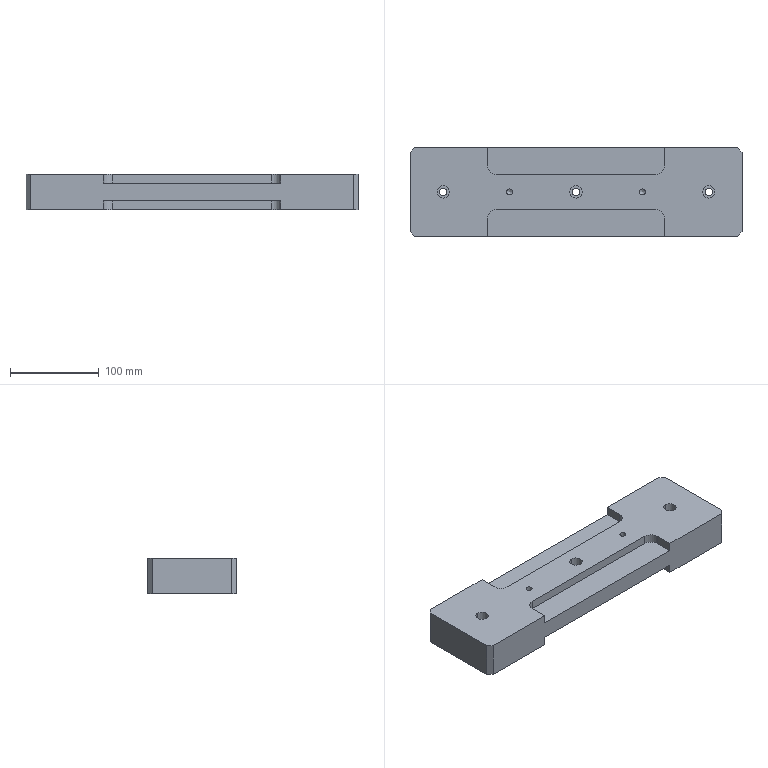NC program | NX | posted with a generic post | part box 375 x 100 x 40 mm
Whole program:
N10 G17 G21 G94 G90
(FLOOR_WALL_COPY , TOOL : D17R0.8)
N12 T21 M6
N14 G54
N16 G17 G0 G90 X6.755 Y-60. S2000 M3
N18 G43 Z30. H21
N20 Z1.17
N22 G94 G1 Z-0.33 F1000.
N24 X1.472 Y-50.85
N26 G3 X0. Y-50. R1.7
N28 G1 X-91.35 F2000.
N30 Y-30.
N32 G2 X-90. Y-28.65 R1.35
N34 G1 X90.
N36 G2 X91.35 Y-30. R1.35
N38 G1 Y-50.
N40 X0.
N42 Y-41.5
N44 X-82.85
N46 Y-37.15
N48 X82.85
N50 Y-41.5
N52 X0.
N54 G3 X-1.472 Y-42.35 R1.7
N56 G1 Z1.17
N58 G0 X6.755 Y-60. Z0.84
N60 G1 Z-0.66 F1000.
N62 X1.472 Y-50.85
N64 G3 X0. Y-50. R1.7
N66 G1 X-91.35 F2000.
N68 Y-30.
N70 G2 X-90. Y-28.65 R1.35
N72 G1 X90.
N74 G2 X91.35 Y-30. R1.35
N76 G1 Y-50.
N78 X0.
N80 Y-41.5
N82 X-82.85
N84 Y-37.15
N86 X82.85
N88 Y-41.5
N90 X0.
N92 G3 X-1.472 Y-42.35 R1.7
N94 G1 Z0.84
N96 G0 X6.755 Y-60. Z0.51
N98 G1 Z-0.99 F1000.
N100 X1.472 Y-50.85
N102 G3 X0. Y-50. R1.7
N104 G1 X-91.35 F2000.
N106 Y-30.
N108 G2 X-90. Y-28.65 R1.35
N110 G1 X90.
N112 G2 X91.35 Y-30. R1.35
N114 G1 Y-50.
N116 X0.
N118 Y-41.5
N120 X-82.85
N122 Y-37.15
N124 X82.85
N126 Y-41.5
N128 X0.
N130 G3 X-1.472 Y-42.35 R1.7
N132 G1 Z0.51
N134 G0 X6.755 Y-60. Z0.18
N136 G1 Z-1.32 F1000.
N138 X1.472 Y-50.85
N140 G3 X0. Y-50. R1.7
N142 G1 X-91.35 F2000.
N144 Y-30.
N146 G2 X-90. Y-28.65 R1.35
N148 G1 X90.
N150 G2 X91.35 Y-30. R1.35
N152 G1 Y-50.
N154 X0.
N156 Y-41.5
N158 X-82.85
N160 Y-37.15
N162 X82.85
N164 Y-41.5
N166 X0.
N168 G3 X-1.472 Y-42.35 R1.7
N170 G1 Z0.18
N172 G0 X6.755 Y-60. Z-0.15
N174 G1 Z-1.65 F1000.
N176 X1.472 Y-50.85
N178 G3 X0. Y-50. R1.7
N180 G1 X-91.35 F2000.
N182 Y-30.
N184 G2 X-90. Y-28.65 R1.35
N186 G1 X90.
N188 G2 X91.35 Y-30. R1.35
N190 G1 Y-50.
N192 X0.
N194 Y-41.5
N196 X-82.85
N198 Y-37.15
N200 X82.85
N202 Y-41.5
N204 X0.
N206 G3 X-1.472 Y-42.35 R1.7
N208 G1 Z-0.15
N210 G0 X6.755 Y-60. Z-0.48
N212 G1 Z-1.98 F1000.
N214 X1.472 Y-50.85
N216 G3 X0. Y-50. R1.7
N218 G1 X-91.35 F2000.
N220 Y-30.
N222 G2 X-90. Y-28.65 R1.35
N224 G1 X90.
N226 G2 X91.35 Y-30. R1.35
N228 G1 Y-50.
N230 X0.
N232 Y-41.5
N234 X-82.85
N236 Y-37.15
N238 X82.85
N240 Y-41.5
N242 X0.
N244 G3 X-1.472 Y-42.35 R1.7
N246 G1 Z-0.48
N248 G0 X6.755 Y-60. Z-0.81
N250 G1 Z-2.31 F1000.
N252 X1.472 Y-50.85
N254 G3 X0. Y-50. R1.7
N256 G1 X-91.35 F2000.
N258 Y-30.
N260 G2 X-90. Y-28.65 R1.35
N262 G1 X90.
N264 G2 X91.35 Y-30. R1.35
N266 G1 Y-50.
N268 X0.
N270 Y-41.5
N272 X-82.85
N274 Y-37.15
N276 X82.85
N278 Y-41.5
N280 X0.
N282 G3 X-1.472 Y-42.35 R1.7
N284 G1 Z-0.81
N286 G0 X6.755 Y-60. Z-1.14
N288 G1 Z-2.64 F1000.
N290 X1.472 Y-50.85
N292 G3 X0. Y-50. R1.7
N294 G1 X-91.35 F2000.
N296 Y-30.
N298 G2 X-90. Y-28.65 R1.35
N300 G1 X90.
N302 G2 X91.35 Y-30. R1.35
N304 G1 Y-50.
N306 X0.
N308 Y-41.5
N310 X-82.85
N312 Y-37.15
N314 X82.85
N316 Y-41.5
N318 X0.
N320 G3 X-1.472 Y-42.35 R1.7
N322 G1 Z-1.14
N324 G0 X6.755 Y-60. Z-1.47
N326 G1 Z-2.97 F1000.
N328 X1.472 Y-50.85
N330 G3 X0. Y-50. R1.7
N332 G1 X-91.35 F2000.
N334 Y-30.
N336 G2 X-90. Y-28.65 R1.35
N338 G1 X90.
N340 G2 X91.35 Y-30. R1.35
N342 G1 Y-50.
N344 X0.
N346 Y-41.5
N348 X-82.85
N350 Y-37.15
N352 X82.85
N354 Y-41.5
N356 X0.
N358 G3 X-1.472 Y-42.35 R1.7
N360 G1 Z-1.47
N362 G0 X6.755 Y-60. Z-1.8
N364 G1 Z-3.3 F1000.
N366 X1.472 Y-50.85
N368 G3 X0. Y-50. R1.7
N370 G1 X-91.35 F2000.
N372 Y-30.
N374 G2 X-90. Y-28.65 R1.35
N376 G1 X90.
N378 G2 X91.35 Y-30. R1.35
N380 G1 Y-50.
N382 X0.
N384 Y-41.5
N386 X-82.85
N388 Y-37.15
N390 X82.85
N392 Y-41.5
N394 X0.
N396 G3 X-1.472 Y-42.35 R1.7
N398 G1 Z-1.8
N400 G0 X6.755 Y-60. Z-2.13
N402 G1 Z-3.63 F1000.
N404 X1.472 Y-50.85
N406 G3 X0. Y-50. R1.7
N408 G1 X-91.35 F2000.
N410 Y-30.
N412 G2 X-90. Y-28.65 R1.35
N414 G1 X90.
N416 G2 X91.35 Y-30. R1.35
N418 G1 Y-50.
N420 X0.
N422 Y-41.5
N424 X-82.85
N426 Y-37.15
N428 X82.85
N430 Y-41.5
N432 X0.
N434 G3 X-1.472 Y-42.35 R1.7
N436 G1 Z-2.13
N438 G0 X6.755 Y-60. Z-2.46
N440 G1 Z-3.96 F1000.
N442 X1.472 Y-50.85
N444 G3 X0. Y-50. R1.7
N446 G1 X-91.35 F2000.
N448 Y-30.
N450 G2 X-90. Y-28.65 R1.35
N452 G1 X90.
N454 G2 X91.35 Y-30. R1.35
N456 G1 Y-50.
N458 X0.
N460 Y-41.5
N462 X-82.85
N464 Y-37.15
N466 X82.85
N468 Y-41.5
N470 X0.
N472 G3 X-1.472 Y-42.35 R1.7
N474 G1 Z-2.46
N476 G0 X6.755 Y-60. Z-2.79
N478 G1 Z-4.29 F1000.
N480 X1.472 Y-50.85
N482 G3 X0. Y-50. R1.7
N484 G1 X-91.35 F2000.
N486 Y-30.
N488 G2 X-90. Y-28.65 R1.35
N490 G1 X90.
N492 G2 X91.35 Y-30. R1.35
N494 G1 Y-50.
N496 X0.
N498 Y-41.5
N500 X-82.85
N502 Y-37.15
N504 X82.85
N506 Y-41.5
N508 X0.
N510 G3 X-1.472 Y-42.35 R1.7
N512 G1 Z-2.79
N514 G0 X6.755 Y-60. Z-3.12
N516 G1 Z-4.62 F1000.
N518 X1.472 Y-50.85
N520 G3 X0. Y-50. R1.7
N522 G1 X-91.35 F2000.
N524 Y-30.
N526 G2 X-90. Y-28.65 R1.35
N528 G1 X90.
N530 G2 X91.35 Y-30. R1.35
N532 G1 Y-50.
N534 X0.
N536 Y-41.5
N538 X-82.85
N540 Y-37.15
N542 X82.85
N544 Y-41.5
N546 X0.
N548 G3 X-1.472 Y-42.35 R1.7
N550 G1 Z-3.12
N552 G0 X6.755 Y-60. Z-3.45
N554 G1 Z-4.95 F1000.
N556 X1.472 Y-50.85
N558 G3 X0. Y-50. R1.7
N560 G1 X-91.35 F2000.
N562 Y-30.
N564 G2 X-90. Y-28.65 R1.35
N566 G1 X90.
N568 G2 X91.35 Y-30. R1.35
N570 G1 Y-50.
N572 X0.
N574 Y-41.5
N576 X-82.85
N578 Y-37.15
N580 X82.85
N582 Y-41.5
N584 X0.
N586 G3 X-1.472 Y-42.35 R1.7
N588 G1 Z-3.45
N590 G0 X6.755 Y-60. Z-3.78
N592 G1 Z-5.28 F1000.
N594 X1.472 Y-50.85
N596 G3 X0. Y-50. R1.7
N598 G1 X-91.35 F2000.
N600 Y-30.
N602 G2 X-90. Y-28.65 R1.35
N604 G1 X90.
N606 G2 X91.35 Y-30. R1.35
N608 G1 Y-50.
N610 X0.
N612 Y-41.5
N614 X-82.85
N616 Y-37.15
N618 X82.85
N620 Y-41.5
N622 X0.
N624 G3 X-1.472 Y-42.35 R1.7
N626 G1 Z-3.78
N628 G0 X6.755 Y-60. Z-4.11
N630 G1 Z-5.61 F1000.
N632 X1.472 Y-50.85
N634 G3 X0. Y-50. R1.7
N636 G1 X-91.35 F2000.
N638 Y-30.
N640 G2 X-90. Y-28.65 R1.35
N642 G1 X90.
N644 G2 X91.35 Y-30. R1.35
N646 G1 Y-50.
N648 X0.
N650 Y-41.5
N652 X-82.85
N654 Y-37.15
N656 X82.85
N658 Y-41.5
N660 X0.
N662 G3 X-1.472 Y-42.35 R1.7
N664 G1 Z-4.11
N666 G0 X6.755 Y-60. Z-4.44
N668 G1 Z-5.94 F1000.
N670 X1.472 Y-50.85
N672 G3 X0. Y-50. R1.7
N674 G1 X-91.35 F2000.
N676 Y-30.
N678 G2 X-90. Y-28.65 R1.35
N680 G1 X90.
N682 G2 X91.35 Y-30. R1.35
N684 G1 Y-50.
N686 X0.
N688 Y-41.5
N690 X-82.85
N692 Y-37.15
N694 X82.85
N696 Y-41.5
N698 X0.
N700 G3 X-1.472 Y-42.35 R1.7
N702 G1 Z-4.44
N704 G0 X6.755 Y-60. Z-4.77
N706 G1 Z-6.27 F1000.
N708 X1.472 Y-50.85
N710 G3 X0. Y-50. R1.7
N712 G1 X-91.35 F2000.
N714 Y-30.
N716 G2 X-90. Y-28.65 R1.35
N718 G1 X90.
N720 G2 X91.35 Y-30. R1.35
N722 G1 Y-50.
N724 X0.
N726 Y-41.5
N728 X-82.85
N730 Y-37.15
N732 X82.85
N734 Y-41.5
N736 X0.
N738 G3 X-1.472 Y-42.35 R1.7
N740 G1 Z-4.77
N742 G0 X6.755 Y-60. Z-5.1
N744 G1 Z-6.6 F1000.
N746 X1.472 Y-50.85
N748 G3 X0. Y-50. R1.7
N750 G1 X-91.35 F2000.
N752 Y-30.
N754 G2 X-90. Y-28.65 R1.35
N756 G1 X90.
N758 G2 X91.35 Y-30. R1.35
N760 G1 Y-50.
N762 X0.
N764 Y-41.5
N766 X-82.85
N768 Y-37.15
N770 X82.85
N772 Y-41.5
N774 X0.
N776 G3 X-1.472 Y-42.35 R1.7
N778 G1 Z-5.1
N780 G0 X6.755 Y-60. Z-5.43
N782 G1 Z-6.93 F1000.
N784 X1.472 Y-50.85
N786 G3 X0. Y-50. R1.7
N788 G1 X-91.35 F2000.
N790 Y-30.
N792 G2 X-90. Y-28.65 R1.35
N794 G1 X90.
N796 G2 X91.35 Y-30. R1.35
N798 G1 Y-50.
N800 X0.
N802 Y-41.5
N804 X-82.85
N806 Y-37.15
N808 X82.85
N810 Y-41.5
N812 X0.
N814 G3 X-1.472 Y-42.35 R1.7
N816 G1 Z-5.43
N818 G0 X6.755 Y-60. Z-5.76
N820 G1 Z-7.26 F1000.
N822 X1.472 Y-50.85
N824 G3 X0. Y-50. R1.7
N826 G1 X-91.35 F2000.
N828 Y-30.
N830 G2 X-90. Y-28.65 R1.35
N832 G1 X90.
N834 G2 X91.35 Y-30. R1.35
N836 G1 Y-50.
N838 X0.
N840 Y-41.5
N842 X-82.85
N844 Y-37.15
N846 X82.85
N848 Y-41.5
N850 X0.
N852 G3 X-1.472 Y-42.35 R1.7
N854 G1 Z-5.76
N856 G0 X6.755 Y-60. Z-6.09
N858 G1 Z-7.59 F1000.
N860 X1.472 Y-50.85
N862 G3 X0. Y-50. R1.7
N864 G1 X-91.35 F2000.
N866 Y-30.
N868 G2 X-90. Y-28.65 R1.35
N870 G1 X90.
N872 G2 X91.35 Y-30. R1.35
N874 G1 Y-50.
N876 X0.
N878 Y-41.5
N880 X-82.85
N882 Y-37.15
N884 X82.85
N886 Y-41.5
N888 X0.
N890 G3 X-1.472 Y-42.35 R1.7
N892 G1 Z-6.09
N894 G0 X6.755 Y-60. Z-6.42
N896 G1 Z-7.92 F1000.
N898 X1.472 Y-50.85
N900 G3 X0. Y-50. R1.7
N902 G1 X-91.35 F2000.
N904 Y-30.
N906 G2 X-90. Y-28.65 R1.35
N908 G1 X90.
N910 G2 X91.35 Y-30. R1.35
N912 G1 Y-50.
N914 X0.
N916 Y-41.5
N918 X-82.85
N920 Y-37.15
N922 X82.85
N924 Y-41.5
N926 X0.
N928 G3 X-1.472 Y-42.35 R1.7
N930 G1 Z-6.42
N932 G0 X6.755 Y-60. Z-6.75
N934 G1 Z-8.25 F1000.
N936 X1.472 Y-50.85
N938 G3 X0. Y-50. R1.7
N940 G1 X-91.35 F2000.
N942 Y-30.
N944 G2 X-90. Y-28.65 R1.35
N946 G1 X90.
N948 G2 X91.35 Y-30. R1.35
N950 G1 Y-50.
N952 X0.
N954 Y-41.5
N956 X-82.85
N958 Y-37.15
N960 X82.85
N962 Y-41.5
N964 X0.
N966 G3 X-1.472 Y-42.35 R1.7
N968 G1 Z-6.75
N970 G0 X6.755 Y-60. Z-7.08
N972 G1 Z-8.58 F1000.
N974 X1.472 Y-50.85
N976 G3 X0. Y-50. R1.7
N978 G1 X-91.35 F2000.
N980 Y-30.
N982 G2 X-90. Y-28.65 R1.35
N984 G1 X90.
N986 G2 X91.35 Y-30. R1.35
N988 G1 Y-50.
N990 X0.
N992 Y-41.5
N994 X-82.85
N996 Y-37.15
N998 X82.85
N1000 Y-41.5
N1002 X0.
N1004 G3 X-1.472 Y-42.35 R1.7
N1006 G1 Z-7.08
N1008 G0 X6.755 Y-60. Z-7.41
N1010 G1 Z-8.91 F1000.
N1012 X1.472 Y-50.85
N1014 G3 X0. Y-50. R1.7
N1016 G1 X-91.35 F2000.
N1018 Y-30.
N1020 G2 X-90. Y-28.65 R1.35
N1022 G1 X90.
N1024 G2 X91.35 Y-30. R1.35
N1026 G1 Y-50.
N1028 X0.
N1030 Y-41.5
N1032 X-82.85
N1034 Y-37.15
N1036 X82.85
N1038 Y-41.5
N1040 X0.
N1042 G3 X-1.472 Y-42.35 R1.7
N1044 G1 Z-7.41
N1046 G0 X6.755 Y-60. Z-7.74
N1048 G1 Z-9.24 F1000.
N1050 X1.472 Y-50.85
N1052 G3 X0. Y-50. R1.7
N1054 G1 X-91.35 F2000.
N1056 Y-30.
N1058 G2 X-90. Y-28.65 R1.35
N1060 G1 X90.
N1062 G2 X91.35 Y-30. R1.35
N1064 G1 Y-50.
N1066 X0.
N1068 Y-41.5
N1070 X-82.85
N1072 Y-37.15
N1074 X82.85
N1076 Y-41.5
N1078 X0.
N1080 G3 X-1.472 Y-42.35 R1.7
N1082 G1 Z-7.74
N1084 G0 X6.755 Y-60. Z-8.07
N1086 G1 Z-9.57 F1000.
N1088 X1.472 Y-50.85
N1090 G3 X0. Y-50. R1.7
N1092 G1 X-91.35 F2000.
N1094 Y-30.
N1096 G2 X-90. Y-28.65 R1.35
N1098 G1 X90.
N1100 G2 X91.35 Y-30. R1.35
N1102 G1 Y-50.
N1104 X0.
N1106 Y-41.5
N1108 X-82.85
N1110 Y-37.15
N1112 X82.85
N1114 Y-41.5
N1116 X0.
N1118 G3 X-1.472 Y-42.35 R1.7
N1120 G1 Z-8.07
N1122 G0 X6.755 Y-60. Z-8.4
N1124 G1 Z-9.9 F1000.
N1126 X1.472 Y-50.85
N1128 G3 X0. Y-50. R1.7
N1130 G1 X-91.35 F2000.
N1132 Y-30.
N1134 G2 X-90. Y-28.65 R1.35
N1136 G1 X90.
N1138 G2 X91.35 Y-30. R1.35
N1140 G1 Y-50.
N1142 X0.
N1144 Y-41.5
N1146 X-82.85
N1148 Y-37.15
N1150 X82.85
N1152 Y-41.5
N1154 X0.
N1156 G3 X-1.472 Y-42.35 R1.7
N1158 G1 Z-8.4
N1160 G0 Z30.
N1162 X-6.755 Y60.
N1164 Z1.17
N1166 G1 Z-0.33 F1000.
N1168 X-1.472 Y50.85
N1170 G3 X0. Y50. R1.7
N1172 G1 X91.35 F2000.
N1174 Y30.
N1176 G2 X90. Y28.65 R1.35
N1178 G1 X-90.
N1180 G2 X-91.35 Y30. R1.35
N1182 G1 Y50.
N1184 X0.
N1186 Y41.5
N1188 X82.85
N1190 Y37.15
N1192 X-82.85
N1194 Y41.5
N1196 X0.
N1198 G3 X1.472 Y42.35 R1.7
N1200 G1 Z1.17
N1202 G0 X-6.755 Y60. Z0.84
N1204 G1 Z-0.66 F1000.
N1206 X-1.472 Y50.85
N1208 G3 X0. Y50. R1.7
N1210 G1 X91.35 F2000.
N1212 Y30.
N1214 G2 X90. Y28.65 R1.35
N1216 G1 X-90.
N1218 G2 X-91.35 Y30. R1.35
N1220 G1 Y50.
N1222 X0.
N1224 Y41.5
N1226 X82.85
N1228 Y37.15
N1230 X-82.85
N1232 Y41.5
N1234 X0.
N1236 G3 X1.472 Y42.35 R1.7
N1238 G1 Z0.84
N1240 G0 X-6.755 Y60. Z0.51
N1242 G1 Z-0.99 F1000.
N1244 X-1.472 Y50.85
N1246 G3 X0. Y50. R1.7
N1248 G1 X91.35 F2000.
N1250 Y30.
N1252 G2 X90. Y28.65 R1.35
N1254 G1 X-90.
N1256 G2 X-91.35 Y30. R1.35
N1258 G1 Y50.
N1260 X0.
N1262 Y41.5
N1264 X82.85
N1266 Y37.15
N1268 X-82.85
N1270 Y41.5
N1272 X0.
N1274 G3 X1.472 Y42.35 R1.7
N1276 G1 Z0.51
N1278 G0 X-6.755 Y60. Z0.18
N1280 G1 Z-1.32 F1000.
N1282 X-1.472 Y50.85
N1284 G3 X0. Y50. R1.7
N1286 G1 X91.35 F2000.
N1288 Y30.
N1290 G2 X90. Y28.65 R1.35
N1292 G1 X-90.
N1294 G2 X-91.35 Y30. R1.35
N1296 G1 Y50.
N1298 X0.
N1300 Y41.5
N1302 X82.85
N1304 Y37.15
N1306 X-82.85
N1308 Y41.5
N1310 X0.
N1312 G3 X1.472 Y42.35 R1.7
N1314 G1 Z0.18
N1316 G0 X-6.755 Y60. Z-0.15
N1318 G1 Z-1.65 F1000.
N1320 X-1.472 Y50.85
N1322 G3 X0. Y50. R1.7
N1324 G1 X91.35 F2000.
N1326 Y30.
N1328 G2 X90. Y28.65 R1.35
N1330 G1 X-90.
N1332 G2 X-91.35 Y30. R1.35
N1334 G1 Y50.
N1336 X0.
N1338 Y41.5
N1340 X82.85
N1342 Y37.15
N1344 X-82.85
N1346 Y41.5
N1348 X0.
N1350 G3 X1.472 Y42.35 R1.7
N1352 G1 Z-0.15
N1354 G0 X-6.755 Y60. Z-0.48
N1356 G1 Z-1.98 F1000.
N1358 X-1.472 Y50.85
N1360 G3 X0. Y50. R1.7
N1362 G1 X91.35 F2000.
N1364 Y30.
N1366 G2 X90. Y28.65 R1.35
N1368 G1 X-90.
N1370 G2 X-91.35 Y30. R1.35
N1372 G1 Y50.
N1374 X0.
N1376 Y41.5
N1378 X82.85
N1380 Y37.15
N1382 X-82.85
N1384 Y41.5
N1386 X0.
N1388 G3 X1.472 Y42.35 R1.7
N1390 G1 Z-0.48
N1392 G0 X-6.755 Y60. Z-0.81
N1394 G1 Z-2.31 F1000.
N1396 X-1.472 Y50.85
N1398 G3 X0. Y50. R1.7
N1400 G1 X91.35 F2000.
N1402 Y30.
N1404 G2 X90. Y28.65 R1.35
N1406 G1 X-90.
N1408 G2 X-91.35 Y30. R1.35
N1410 G1 Y50.
N1412 X0.
N1414 Y41.5
N1416 X82.85
N1418 Y37.15
N1420 X-82.85
N1422 Y41.5
N1424 X0.
N1426 G3 X1.472 Y42.35 R1.7
N1428 G1 Z-0.81
N1430 G0 X-6.755 Y60. Z-1.14
N1432 G1 Z-2.64 F1000.
N1434 X-1.472 Y50.85
N1436 G3 X0. Y50. R1.7
N1438 G1 X91.35 F2000.
N1440 Y30.
N1442 G2 X90. Y28.65 R1.35
N1444 G1 X-90.
N1446 G2 X-91.35 Y30. R1.35
N1448 G1 Y50.
N1450 X0.
N1452 Y41.5
N1454 X82.85
N1456 Y37.15
N1458 X-82.85
N1460 Y41.5
N1462 X0.
N1464 G3 X1.472 Y42.35 R1.7
N1466 G1 Z-1.14
N1468 G0 X-6.755 Y60. Z-1.47
N1470 G1 Z-2.97 F1000.
N1472 X-1.472 Y50.85
N1474 G3 X0. Y50. R1.7
N1476 G1 X91.35 F2000.
N1478 Y30.
N1480 G2 X90. Y28.65 R1.35
N1482 G1 X-90.
N1484 G2 X-91.35 Y30. R1.35
N1486 G1 Y50.
N1488 X0.
N1490 Y41.5
N1492 X82.85
N1494 Y37.15
N1496 X-82.85
N1498 Y41.5
N1500 X0.
N1502 G3 X1.472 Y42.35 R1.7
N1504 G1 Z-1.47
N1506 G0 X-6.755 Y60. Z-1.8
N1508 G1 Z-3.3 F1000.
N1510 X-1.472 Y50.85
N1512 G3 X0. Y50. R1.7
N1514 G1 X91.35 F2000.
N1516 Y30.
N1518 G2 X90. Y28.65 R1.35
N1520 G1 X-90.
N1522 G2 X-91.35 Y30. R1.35
N1524 G1 Y50.
N1526 X0.
N1528 Y41.5
N1530 X82.85
N1532 Y37.15
N1534 X-82.85
N1536 Y41.5
N1538 X0.
N1540 G3 X1.472 Y42.35 R1.7
N1542 G1 Z-1.8
N1544 G0 X-6.755 Y60. Z-2.13
N1546 G1 Z-3.63 F1000.
N1548 X-1.472 Y50.85
N1550 G3 X0. Y50. R1.7
N1552 G1 X91.35 F2000.
N1554 Y30.
N1556 G2 X90. Y28.65 R1.35
N1558 G1 X-90.
N1560 G2 X-91.35 Y30. R1.35
N1562 G1 Y50.
N1564 X0.
N1566 Y41.5
N1568 X82.85
N1570 Y37.15
N1572 X-82.85
N1574 Y41.5
N1576 X0.
N1578 G3 X1.472 Y42.35 R1.7
N1580 G1 Z-2.13
N1582 G0 X-6.755 Y60. Z-2.46
N1584 G1 Z-3.96 F1000.
N1586 X-1.472 Y50.85
N1588 G3 X0. Y50. R1.7
N1590 G1 X91.35 F2000.
N1592 Y30.
N1594 G2 X90. Y28.65 R1.35
N1596 G1 X-90.
N1598 G2 X-91.35 Y30. R1.35
N1600 G1 Y50.
N1602 X0.
N1604 Y41.5
N1606 X82.85
N1608 Y37.15
N1610 X-82.85
N1612 Y41.5
N1614 X0.
N1616 G3 X1.472 Y42.35 R1.7
N1618 G1 Z-2.46
N1620 G0 X-6.755 Y60. Z-2.79
N1622 G1 Z-4.29 F1000.
N1624 X-1.472 Y50.85
N1626 G3 X0. Y50. R1.7
N1628 G1 X91.35 F2000.
N1630 Y30.
N1632 G2 X90. Y28.65 R1.35
N1634 G1 X-90.
N1636 G2 X-91.35 Y30. R1.35
N1638 G1 Y50.
N1640 X0.
N1642 Y41.5
N1644 X82.85
N1646 Y37.15
N1648 X-82.85
N1650 Y41.5
N1652 X0.
N1654 G3 X1.472 Y42.35 R1.7
N1656 G1 Z-2.79
N1658 G0 X-6.755 Y60. Z-3.12
N1660 G1 Z-4.62 F1000.
N1662 X-1.472 Y50.85
N1664 G3 X0. Y50. R1.7
N1666 G1 X91.35 F2000.
N1668 Y30.
N1670 G2 X90. Y28.65 R1.35
N1672 G1 X-90.
N1674 G2 X-91.35 Y30. R1.35
N1676 G1 Y50.
N1678 X0.
N1680 Y41.5
N1682 X82.85
N1684 Y37.15
N1686 X-82.85
N1688 Y41.5
N1690 X0.
N1692 G3 X1.472 Y42.35 R1.7
N1694 G1 Z-3.12
N1696 G0 X-6.755 Y60. Z-3.45
N1698 G1 Z-4.95 F1000.
N1700 X-1.472 Y50.85
N1702 G3 X0. Y50. R1.7
N1704 G1 X91.35 F2000.
N1706 Y30.
N1708 G2 X90. Y28.65 R1.35
N1710 G1 X-90.
N1712 G2 X-91.35 Y30. R1.35
N1714 G1 Y50.
N1716 X0.
N1718 Y41.5
N1720 X82.85
N1722 Y37.15
N1724 X-82.85
N1726 Y41.5
N1728 X0.
N1730 G3 X1.472 Y42.35 R1.7
N1732 G1 Z-3.45
N1734 G0 X-6.755 Y60. Z-3.78
N1736 G1 Z-5.28 F1000.
N1738 X-1.472 Y50.85
N1740 G3 X0. Y50. R1.7
N1742 G1 X91.35 F2000.
N1744 Y30.
N1746 G2 X90. Y28.65 R1.35
N1748 G1 X-90.
N1750 G2 X-91.35 Y30. R1.35
N1752 G1 Y50.
N1754 X0.
N1756 Y41.5
N1758 X82.85
N1760 Y37.15
N1762 X-82.85
N1764 Y41.5
N1766 X0.
N1768 G3 X1.472 Y42.35 R1.7
N1770 G1 Z-3.78
N1772 G0 X-6.755 Y60. Z-4.11
N1774 G1 Z-5.61 F1000.
N1776 X-1.472 Y50.85
N1778 G3 X0. Y50. R1.7
N1780 G1 X91.35 F2000.
N1782 Y30.
N1784 G2 X90. Y28.65 R1.35
N1786 G1 X-90.
N1788 G2 X-91.35 Y30. R1.35
N1790 G1 Y50.
N1792 X0.
N1794 Y41.5
N1796 X82.85
N1798 Y37.15
N1800 X-82.85
N1802 Y41.5
N1804 X0.
N1806 G3 X1.472 Y42.35 R1.7
N1808 G1 Z-4.11
N1810 G0 X-6.755 Y60. Z-4.44
N1812 G1 Z-5.94 F1000.
N1814 X-1.472 Y50.85
N1816 G3 X0. Y50. R1.7
N1818 G1 X91.35 F2000.
N1820 Y30.
N1822 G2 X90. Y28.65 R1.35
N1824 G1 X-90.
N1826 G2 X-91.35 Y30. R1.35
N1828 G1 Y50.
N1830 X0.
N1832 Y41.5
N1834 X82.85
N1836 Y37.15
N1838 X-82.85
N1840 Y41.5
N1842 X0.
N1844 G3 X1.472 Y42.35 R1.7
N1846 G1 Z-4.44
N1848 G0 X-6.755 Y60. Z-4.77
N1850 G1 Z-6.27 F1000.
N1852 X-1.472 Y50.85
N1854 G3 X0. Y50. R1.7
N1856 G1 X91.35 F2000.
N1858 Y30.
N1860 G2 X90. Y28.65 R1.35
N1862 G1 X-90.
N1864 G2 X-91.35 Y30. R1.35
N1866 G1 Y50.
N1868 X0.
N1870 Y41.5
N1872 X82.85
N1874 Y37.15
N1876 X-82.85
N1878 Y41.5
N1880 X0.
N1882 G3 X1.472 Y42.35 R1.7
N1884 G1 Z-4.77
N1886 G0 X-6.755 Y60. Z-5.1
N1888 G1 Z-6.6 F1000.
N1890 X-1.472 Y50.85
N1892 G3 X0. Y50. R1.7
N1894 G1 X91.35 F2000.
N1896 Y30.
N1898 G2 X90. Y28.65 R1.35
N1900 G1 X-90.
N1902 G2 X-91.35 Y30. R1.35
N1904 G1 Y50.
N1906 X0.
N1908 Y41.5
N1910 X82.85
N1912 Y37.15
N1914 X-82.85
N1916 Y41.5
N1918 X0.
N1920 G3 X1.472 Y42.35 R1.7
N1922 G1 Z-5.1
N1924 G0 X-6.755 Y60. Z-5.43
N1926 G1 Z-6.93 F1000.
N1928 X-1.472 Y50.85
N1930 G3 X0. Y50. R1.7
N1932 G1 X91.35 F2000.
N1934 Y30.
N1936 G2 X90. Y28.65 R1.35
N1938 G1 X-90.
N1940 G2 X-91.35 Y30. R1.35
N1942 G1 Y50.
N1944 X0.
N1946 Y41.5
N1948 X82.85
N1950 Y37.15
N1952 X-82.85
N1954 Y41.5
N1956 X0.
N1958 G3 X1.472 Y42.35 R1.7
N1960 G1 Z-5.43
N1962 G0 X-6.755 Y60. Z-5.76
N1964 G1 Z-7.26 F1000.
N1966 X-1.472 Y50.85
N1968 G3 X0. Y50. R1.7
N1970 G1 X91.35 F2000.
N1972 Y30.
N1974 G2 X90. Y28.65 R1.35
N1976 G1 X-90.
N1978 G2 X-91.35 Y30. R1.35
N1980 G1 Y50.
N1982 X0.
N1984 Y41.5
N1986 X82.85
N1988 Y37.15
N1990 X-82.85
N1992 Y41.5
N1994 X0.
N1996 G3 X1.472 Y42.35 R1.7
N1998 G1 Z-5.76
N2000 G0 X-6.755 Y60. Z-6.09
N2002 G1 Z-7.59 F1000.
N2004 X-1.472 Y50.85
N2006 G3 X0. Y50. R1.7
N2008 G1 X91.35 F2000.
N2010 Y30.
N2012 G2 X90. Y28.65 R1.35
N2014 G1 X-90.
N2016 G2 X-91.35 Y30. R1.35
N2018 G1 Y50.
N2020 X0.
N2022 Y41.5
N2024 X82.85
N2026 Y37.15
N2028 X-82.85
N2030 Y41.5
N2032 X0.
N2034 G3 X1.472 Y42.35 R1.7
N2036 G1 Z-6.09
N2038 G0 X-6.755 Y60. Z-6.42
N2040 G1 Z-7.92 F1000.
N2042 X-1.472 Y50.85
N2044 G3 X0. Y50. R1.7
N2046 G1 X91.35 F2000.
N2048 Y30.
N2050 G2 X90. Y28.65 R1.35
N2052 G1 X-90.
N2054 G2 X-91.35 Y30. R1.35
N2056 G1 Y50.
N2058 X0.
N2060 Y41.5
N2062 X82.85
N2064 Y37.15
N2066 X-82.85
N2068 Y41.5
N2070 X0.
N2072 G3 X1.472 Y42.35 R1.7
N2074 G1 Z-6.42
N2076 G0 X-6.755 Y60. Z-6.75
N2078 G1 Z-8.25 F1000.
N2080 X-1.472 Y50.85
N2082 G3 X0. Y50. R1.7
N2084 G1 X91.35 F2000.
N2086 Y30.
N2088 G2 X90. Y28.65 R1.35
N2090 G1 X-90.
N2092 G2 X-91.35 Y30. R1.35
N2094 G1 Y50.
N2096 X0.
N2098 Y41.5
N2100 X82.85
N2102 Y37.15
N2104 X-82.85
N2106 Y41.5
N2108 X0.
N2110 G3 X1.472 Y42.35 R1.7
N2112 G1 Z-6.75
N2114 G0 X-6.755 Y60. Z-7.08
N2116 G1 Z-8.58 F1000.
N2118 X-1.472 Y50.85
N2120 G3 X0. Y50. R1.7
N2122 G1 X91.35 F2000.
N2124 Y30.
N2126 G2 X90. Y28.65 R1.35
N2128 G1 X-90.
N2130 G2 X-91.35 Y30. R1.35
N2132 G1 Y50.
N2134 X0.
N2136 Y41.5
N2138 X82.85
N2140 Y37.15
N2142 X-82.85
N2144 Y41.5
N2146 X0.
N2148 G3 X1.472 Y42.35 R1.7
N2150 G1 Z-7.08
N2152 G0 X-6.755 Y60. Z-7.41
N2154 G1 Z-8.91 F1000.
N2156 X-1.472 Y50.85
N2158 G3 X0. Y50. R1.7
N2160 G1 X91.35 F2000.
N2162 Y30.
N2164 G2 X90. Y28.65 R1.35
N2166 G1 X-90.
N2168 G2 X-91.35 Y30. R1.35
N2170 G1 Y50.
N2172 X0.
N2174 Y41.5
N2176 X82.85
N2178 Y37.15
N2180 X-82.85
N2182 Y41.5
N2184 X0.
N2186 G3 X1.472 Y42.35 R1.7
N2188 G1 Z-7.41
N2190 G0 X-6.755 Y60. Z-7.74
N2192 G1 Z-9.24 F1000.
N2194 X-1.472 Y50.85
N2196 G3 X0. Y50. R1.7
N2198 G1 X91.35 F2000.
N2200 Y30.
N2202 G2 X90. Y28.65 R1.35
N2204 G1 X-90.
N2206 G2 X-91.35 Y30. R1.35
N2208 G1 Y50.
N2210 X0.
N2212 Y41.5
N2214 X82.85
N2216 Y37.15
N2218 X-82.85
N2220 Y41.5
N2222 X0.
N2224 G3 X1.472 Y42.35 R1.7
N2226 G1 Z-7.74
N2228 G0 X-6.755 Y60. Z-8.07
N2230 G1 Z-9.57 F1000.
N2232 X-1.472 Y50.85
N2234 G3 X0. Y50. R1.7
N2236 G1 X91.35 F2000.
N2238 Y30.
N2240 G2 X90. Y28.65 R1.35
N2242 G1 X-90.
N2244 G2 X-91.35 Y30. R1.35
N2246 G1 Y50.
N2248 X0.
N2250 Y41.5
N2252 X82.85
N2254 Y37.15
N2256 X-82.85
N2258 Y41.5
N2260 X0.
N2262 G3 X1.472 Y42.35 R1.7
N2264 G1 Z-8.07
N2266 G0 X-6.755 Y60. Z-8.4
N2268 G1 Z-9.9 F1000.
N2270 X-1.472 Y50.85
N2272 G3 X0. Y50. R1.7
N2274 G1 X91.35 F2000.
N2276 Y30.
N2278 G2 X90. Y28.65 R1.35
N2280 G1 X-90.
N2282 G2 X-91.35 Y30. R1.35
N2284 G1 Y50.
N2286 X0.
N2288 Y41.5
N2290 X82.85
N2292 Y37.15
N2294 X-82.85
N2296 Y41.5
N2298 X0.
N2300 G3 X1.472 Y42.35 R1.7
N2302 G1 Z-8.4
N2304 G0 Z30.
N2306 M5
(FLOOR_WALL_1_1_COPY_COPY , TOOL : D10JING)
N2308 T11 M6
N2310 G54
N2312 G17 G0 G90 X93.634 Y-55.5 S7000 M3
N2314 G43 Z30. H11
N2316 Z-9.
N2318 G94 G1 Z-10. F1000.
N2320 Y-54.5
N2322 G3 X94.5 Y-55. R1.
N2324 G1 X-94.5
N2326 Y-50.083
N2328 X94.5
N2330 Y-45.167
N2332 X-94.5
N2334 Y-40.25
N2336 X94.5
N2338 Y-35.333
N2340 X-94.5
N2342 Y-30.417
N2344 X94.5
N2346 Y-30.
N2348 G3 X90.015 Y-25.5 R4.5
N2350 G1 X-90.015
N2352 G3 X-90.881 Y-26. R1.
N2354 G1 Z-9.
N2356 G0 Z30.
N2358 X94.5 Y-55.866
N2360 Z-9.
N2362 G1 Z-10.
N2364 G3 X95. Y-55. R1.
N2366 G1 Y-30.
N2368 G3 X90. Y-25. R5.
N2370 G1 X-90.
N2372 G3 X-95. Y-30. R5.
N2374 G1 Y-55.
N2376 G3 X-94.5 Y-55.866 R1.
N2378 G1 Z-9.
N2380 G0 Z30.
N2382 X-93.634 Y55.5
N2384 Z-9.
N2386 G1 Z-10.
N2388 Y54.5
N2390 G3 X-94.5 Y55. R1.
N2392 G1 X94.5
N2394 Y50.083
N2396 X-94.5
N2398 Y45.167
N2400 X94.5
N2402 Y40.25
N2404 X-94.5
N2406 Y35.333
N2408 X94.5
N2410 Y30.417
N2412 X-94.5
N2414 Y30.
N2416 G3 X-90.015 Y25.5 R4.5
N2418 G1 X90.015
N2420 G3 X90.881 Y26. R1.
N2422 G1 Z-9.
N2424 G0 Z30.
N2426 X-94.5 Y55.866
N2428 Z-9.
N2430 G1 Z-10.
N2432 G3 X-95. Y55. R1.
N2434 G1 Y30.
N2436 G3 X-90. Y25. R5.
N2438 G1 X90.
N2440 G3 X95. Y30. R5.
N2442 G1 Y55.
N2444 G3 X94.5 Y55.866 R1.
N2446 G1 Z-9.
N2448 G0 Z30.
N2450 M5
(ZLEVEL_PROFILE_1_COPY_1_COPY_COPY_COPY_1 , TOOL : D6A45)
N2452 T22 M6
N2454 G54
N2456 G17 G0 G90 X1.302 Y1.637 S7500 M3
N2458 G43 Z30. H22
N2460 Z0.
N2462 G94 G1 Z-1. F1000.
N2464 X0.52 Y2.991
N2466 G3 X0. Y3.291 R0.6
N2468 G1 X-0.008
N2470 G3 X-3.291 Y-0.008 R3.291
N2472 X0. Y3.291 R-3.291
N2474 X-0.52 Y2.991 R0.6
N2476 G1 X-1.302 Y1.637
N2478 Z0.
N2480 G0 Z30.
N2482 X-151.637 Y1.302
N2484 Z0.
N2486 G1 Z-1.
N2488 X-152.991 Y0.52
N2490 G3 X-153.291 Y0. R0.6
N2492 X-150. Y-3.291 R3.291
N2494 X-153.291 Y0. R-3.291
N2496 X-152.991 Y-0.52 R0.6
N2498 G1 X-151.637 Y-1.302
N2500 Z0.
N2502 G0 Z30.
N2504 X151.637
N2506 Z0.
N2508 G1 Z-1.
N2510 X152.991 Y-0.52
N2512 G3 X153.291 Y0. R0.6
N2514 X150. Y3.291 R3.291
N2516 X153.291 Y0. R-3.291
N2518 X152.991 Y0.52 R0.6
N2520 G1 X151.637 Y1.302
N2522 Z0.
N2524 G0 Z30.
N2526 X-91.083 Y22.234
N2528 Z0.
N2530 G1 Z-1.
N2532 X-90.52 Y21.259
N2534 G3 X-90. Y20.959 R0.6
N2536 G1 X90.
N2538 G3 X99.041 Y30. R9.041
N2540 G1 Y50.001
N2542 G2 X99.999 Y50.959 R0.967
N2544 G1 X182.501
N2546 G2 X183.177 Y50.678 R0.957
N2548 G1 X188.178 Y45.677
N2550 G2 X188.459 Y45.001 R0.956
N2552 G1 Y-45.001
N2554 G2 X188.178 Y-45.677 R0.956
N2556 G1 X183.177 Y-50.678
N2558 G2 X182.501 Y-50.959 R0.957
N2560 G1 X99.999
N2562 G2 X99.041 Y-50.001 R0.967
N2564 G1 Y-30.
N2566 G3 X90. Y-20.959 R9.041
N2568 G1 X-90.
N2570 G3 X-99.041 Y-30. R9.041
N2572 G1 Y-50.001
N2574 G2 X-99.999 Y-50.959 R0.967
N2576 G1 X-182.501
N2578 G2 X-183.177 Y-50.678 R0.957
N2580 G1 X-188.178 Y-45.677
N2582 G2 X-188.459 Y-45.001 R0.956
N2584 G1 Y45.001
N2586 G2 X-188.178 Y45.677 R0.956
N2588 G1 X-183.177 Y50.678
N2590 G2 X-182.501 Y50.959 R0.957
N2592 G1 X-99.999
N2594 G2 X-99.041 Y50.001 R0.967
N2596 G1 Y30.
N2598 G3 X-90. Y20.959 R9.041
N2600 X-89.48 Y21.259 R0.6
N2602 G1 X-88.961 Y22.159
N2604 Z0.
N2606 G0 Z30.
(ZLEVEL_PROFILE_1_COPY_1_COPY_COPY_COPY_COPY , TOOL : D6A45)
N2608 X96.427 Y-52.159
N2610 Z-10.
N2612 G1 Z-11.
N2614 X96.939 Y-51.549
N2616 G3 X97.043 Y-50.959 R0.6
N2618 G1 X-97.043
N2620 G3 X-96.939 Y-51.549 R0.6
N2622 G1 X-96.427 Y-52.159
N2624 Z-10.
N2626 G0 Z30.
N2628 Y52.159
N2630 Z-10.
N2632 G1 Z-11.
N2634 X-96.939 Y51.549
N2636 G3 X-97.043 Y50.959 R0.6
N2638 G1 X97.043
N2640 G3 X96.939 Y51.549 R0.6
N2642 G1 X96.428 Y52.159
N2644 Z-10.
N2646 G0 Z30.
N2648 M5
N2650 M2